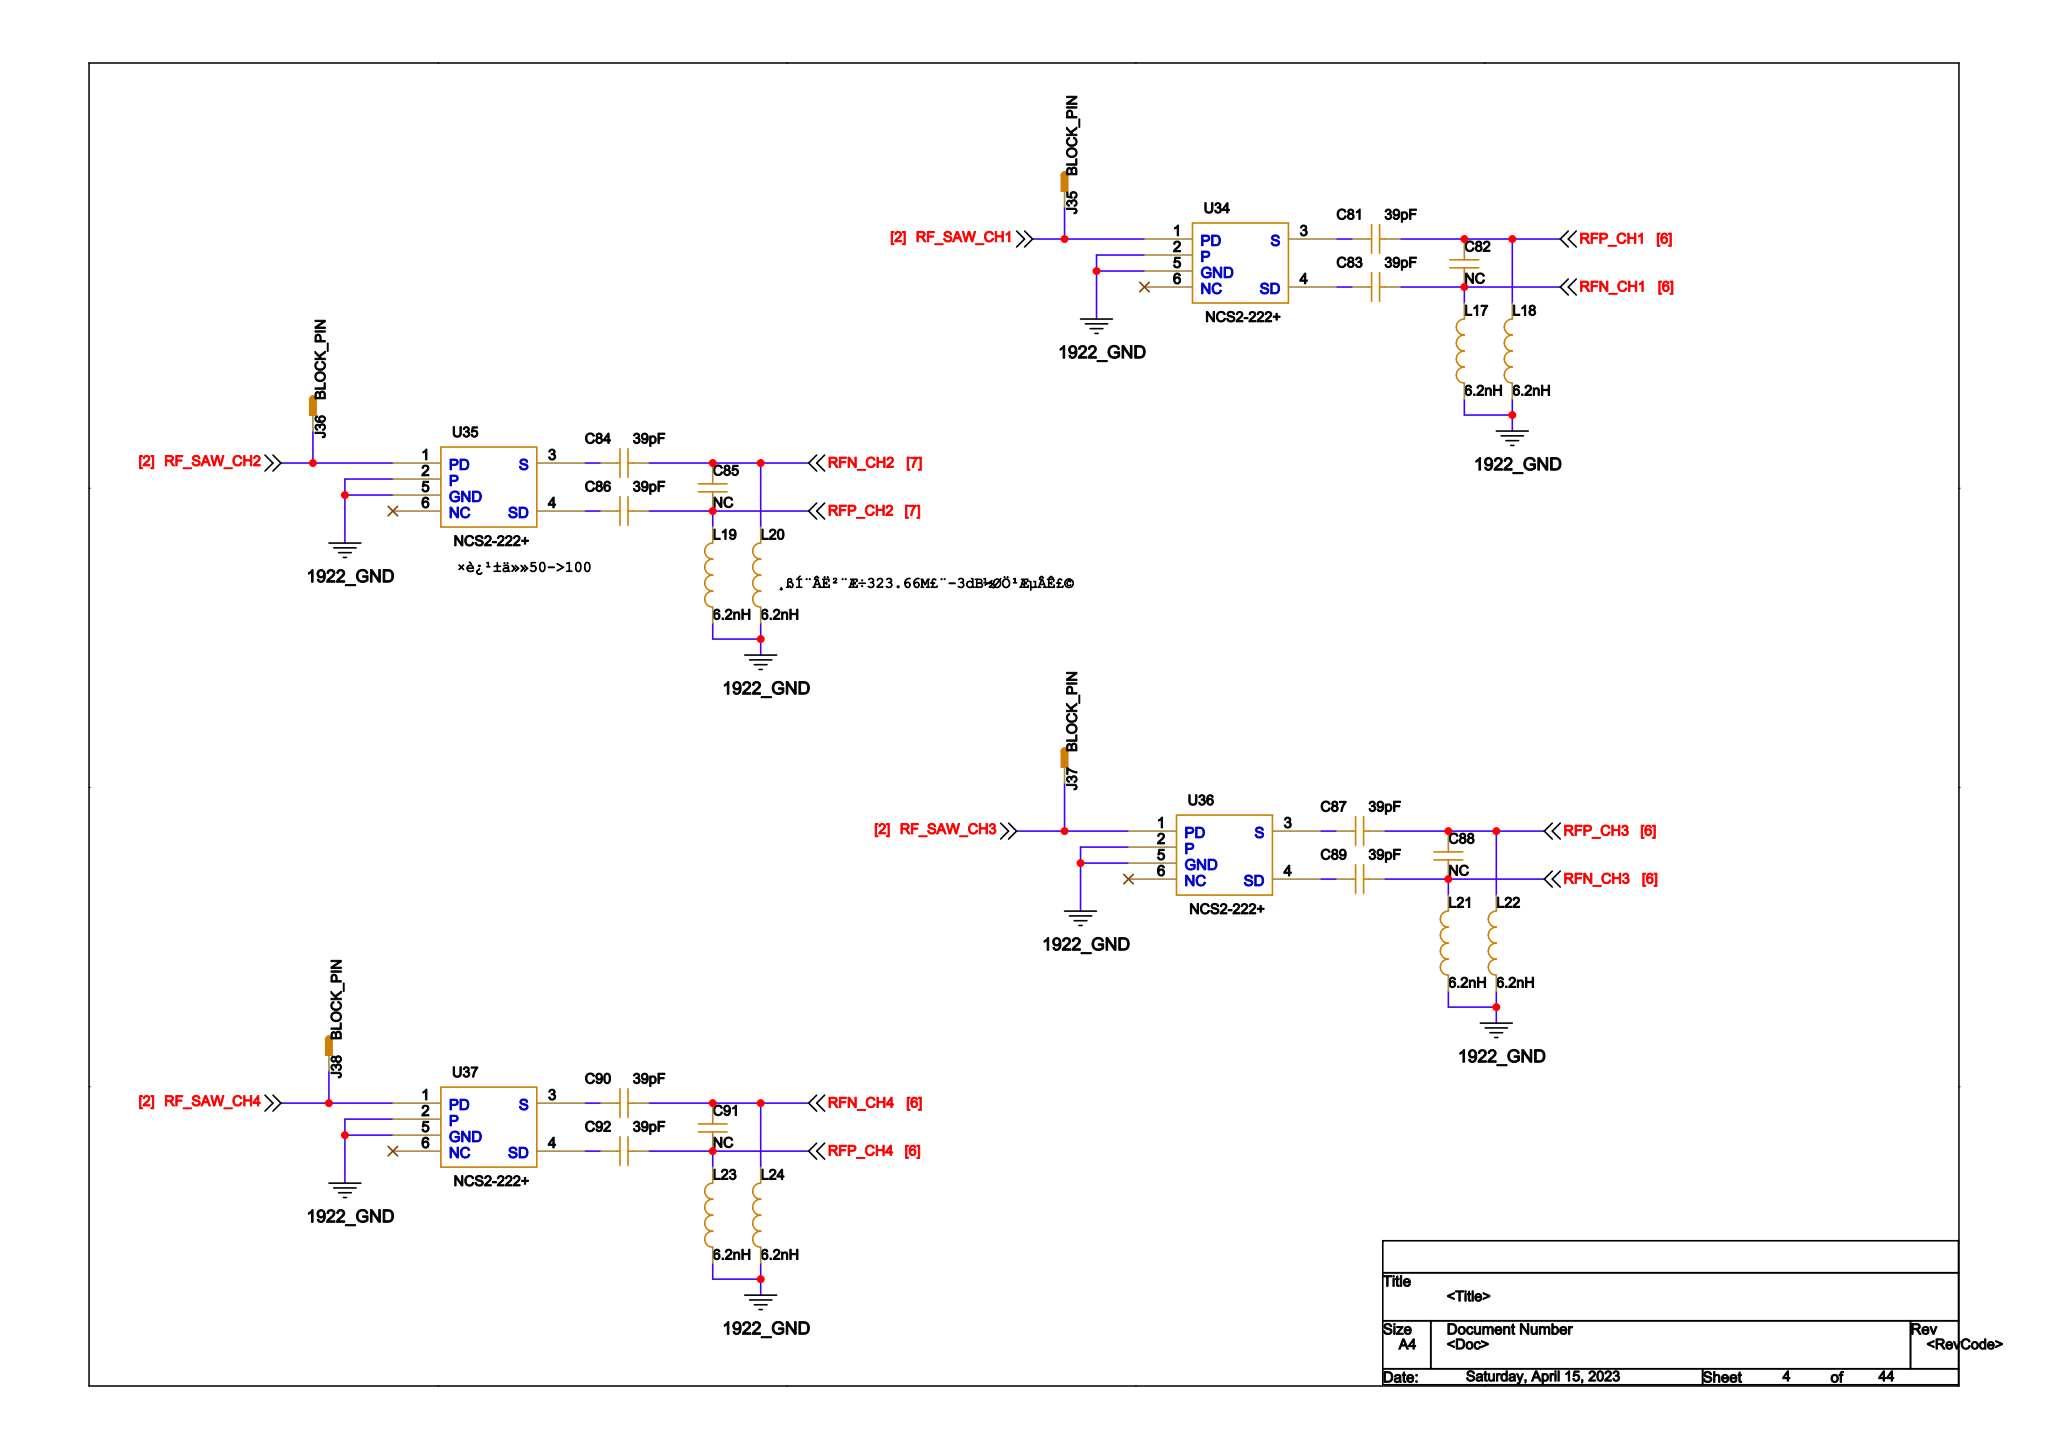Circuit board | Cadence Allegro | 1034 parts | 912 nets | one sheet of the schematic
Parts on this sheet (reference | value | footprint):
C81 | 39pF | C0402
C82 | NC | C0402
C83 | 39pF | C0402
C84 | 39pF | C0402
C85 | NC | C0402
C86 | 39pF | C0402
C87 | 39pF | C0402
C88 | NC | C0402
C89 | 39pF | C0402
C90 | 39pF | C0402
C91 | NC | C0402
C92 | 39pF | C0402
J35 | BLOCK_PIN | B_PIN_SMD
J36 | BLOCK_PIN | B_PIN_SMD
J37 | BLOCK_PIN | B_PIN_SMD
J38 | BLOCK_PIN | B_PIN_SMD
L17 | 6.2nH | L0402
L18 | 6.2nH | L0402
L19 | 6.2nH | L0402
L20 | 6.2nH | L0402
L21 | 6.2nH | L0402
L22 | 6.2nH | L0402
L23 | 6.2nH | L0402
L24 | 6.2nH | L0402
U34 | NCS2-222+ | NCS2_BL_SMD
U35 | NCS2-222+ | NCS2_BL_SMD
U36 | NCS2-222+ | NCS2_BL_SMD
U37 | NCS2-222+ | NCS2_BL_SMD
Nets of these parts (net: part-pin ...):
RF_SAW_CH1_D1: J35-1 U34-1
RF_SAW_CH2_D1: J36-1 U35-1
RF_SAW_CH3_D1: J37-1 U36-1
RF_SAW_CH4_D1: J38-1 U37-1
1922_GND: L17-1 L18-1 L19-1 L20-1 L21-1 L22-1 L23-1 L24-1 U34-2 U34-5 U35-2 U35-5 U36-2 U36-5 U37-2 U37-5
RFN_CH1_D1: C82-1 C83-2 L17-2
RFP_CH1_D1: C81-2 C82-2 L18-2
RFP_CH2_D1: C85-1 C86-2 L19-2
RFN_CH2_D1: C84-2 C85-2 L20-2
RFN_CH3_D1: C88-1 C89-2 L21-2
RFP_CH3_D1: C87-2 C88-2 L22-2
RFP_CH4_D1: C91-1 C92-2 L23-2
RFN_CH4_D1: C90-2 C91-2 L24-2
N435308_D1: C81-1 U34-3
N149989_D1: C83-1 U34-4
N435961_D1: C84-1 U35-3
N436057_D1: C86-1 U35-4
N437474_D1: C87-1 U36-3
N437570_D1: C89-1 U36-4
N436601_D1: C90-1 U37-3
N436697_D1: C92-1 U37-4